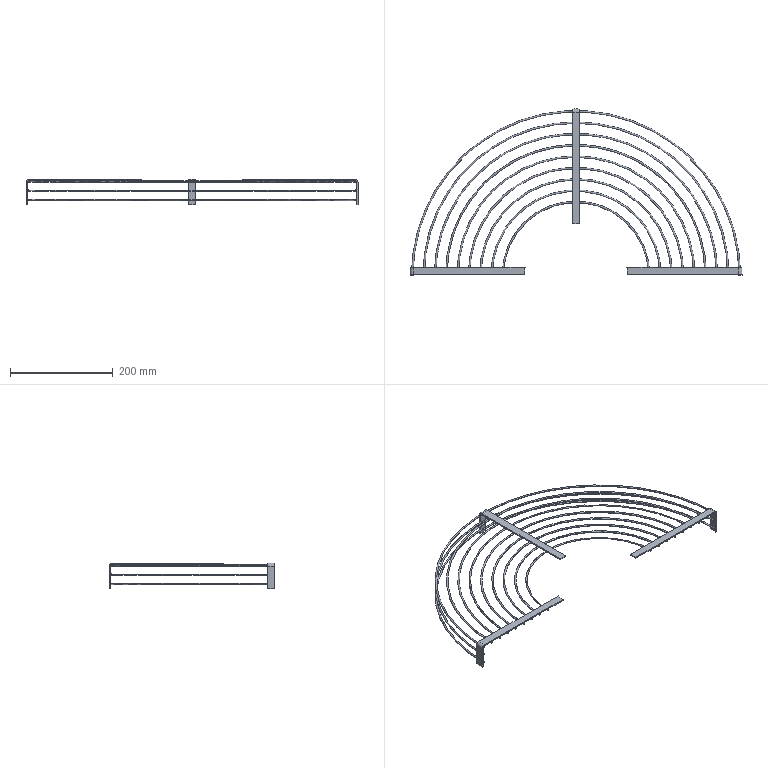Part | STEP file | Produce dryer HY-40-M-021 | 11 solids | 75 faces | box 645 x 322.5 x 50 mm | volume 90254 mm3 | plane 35 | torus 31 | cylinder 9 | commonest cylinder face diameters 200 x3 640 x3 645 x3